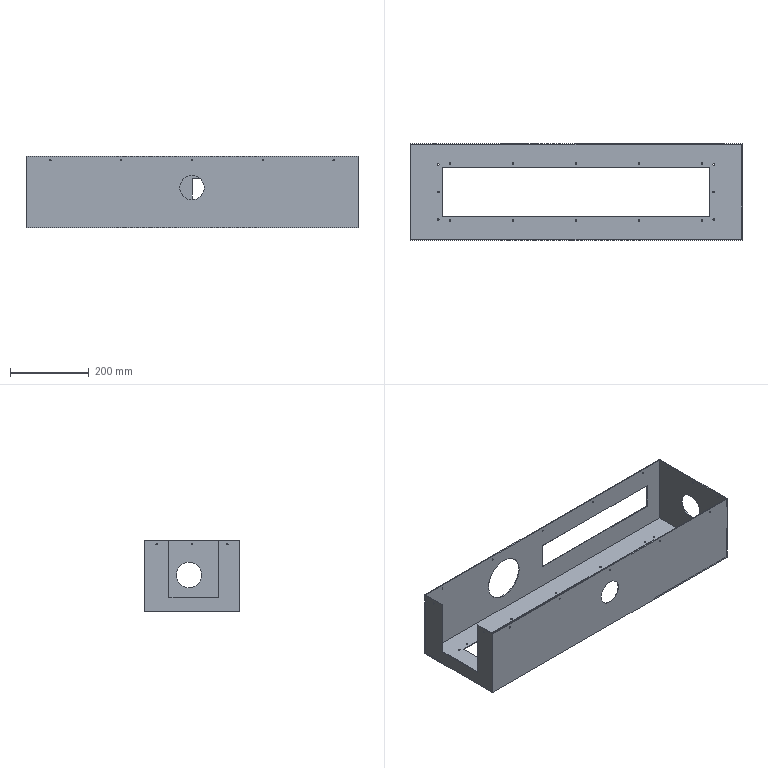Part | NX | features BREP 1 | 1 solid | 90 faces | box 844 x 244 x 182 mm | volume 903231 mm3 | cylinder 68 | plane 22 | commonest cylinder face diameters 4.2 x32 3.3 x30 62 x2 65 x2 110 x2